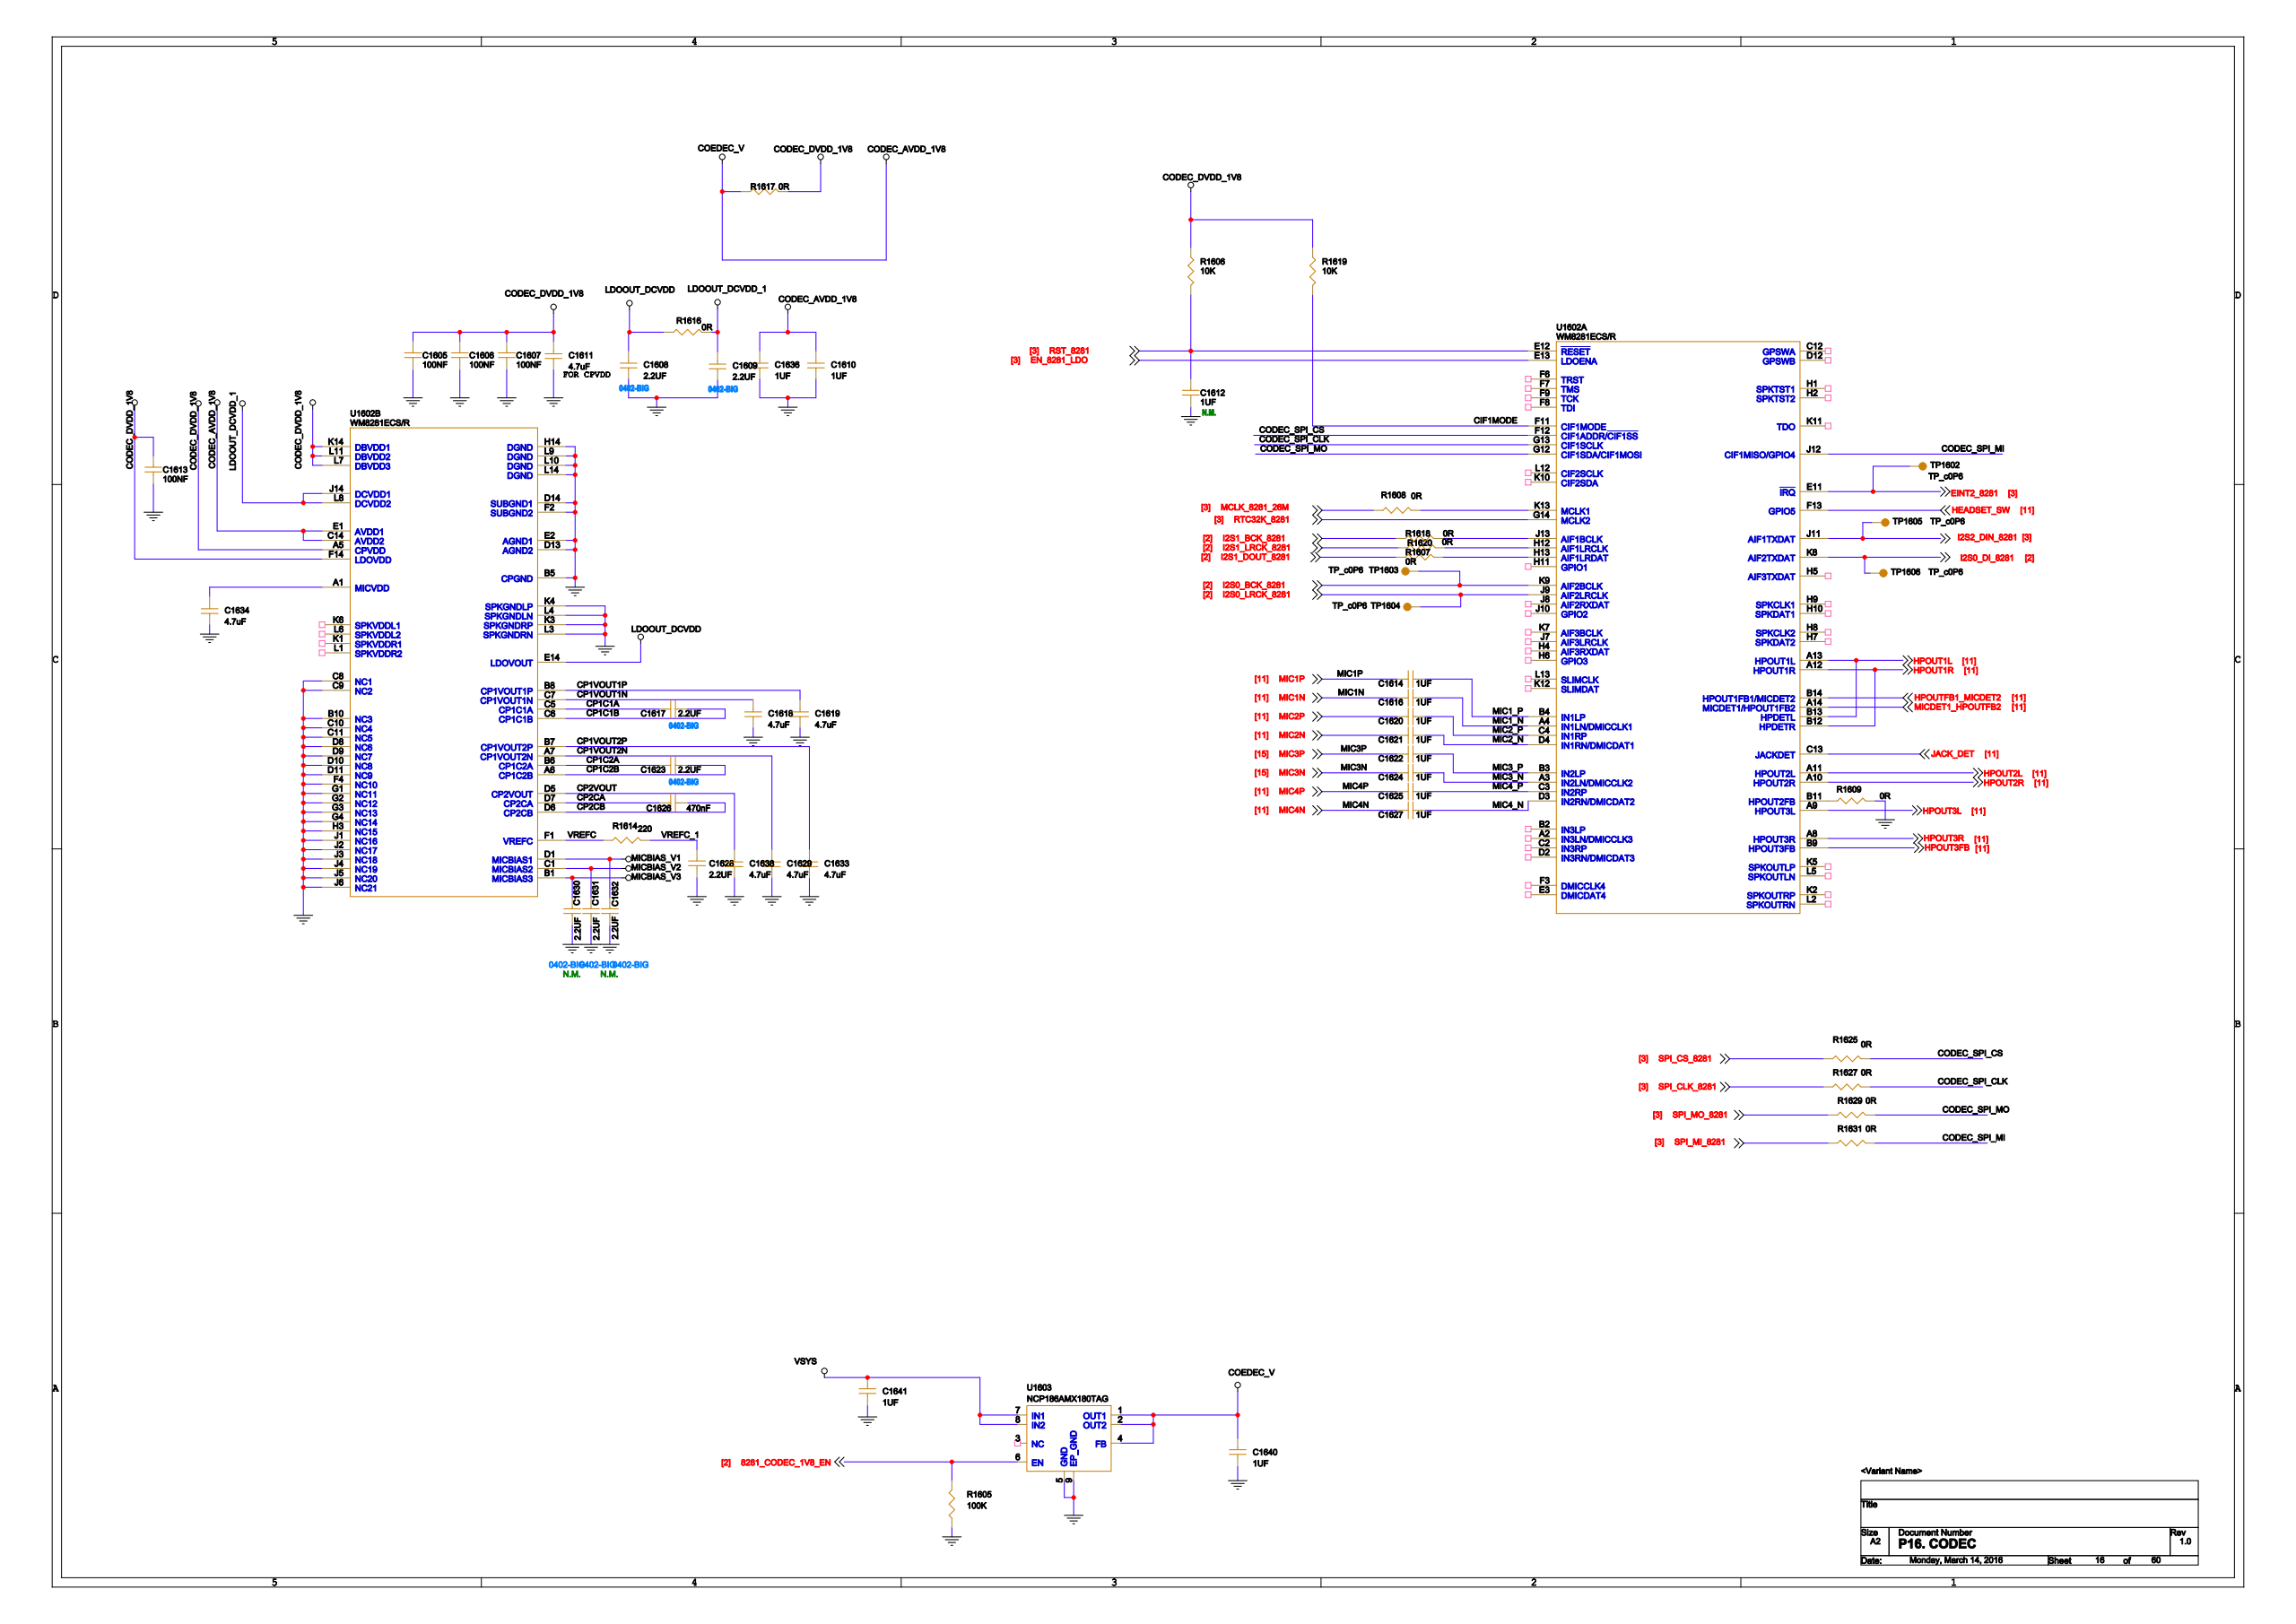Circuit board | Cadence Allegro | 1088 parts | 793 nets | one sheet of the schematic
Parts on this sheet (reference | value | footprint):
C1605 | 100NF | C0201
C1606 | 100NF | C0201
C1607 | 100NF | C0201
C1608 | 2.2UF | 0402-BIG
C1609 | 2.2UF | 0402-BIG
C1610 | 1UF | C0201
C1611 | 4.7uF | 0402-BIG
C1612
C1613 | 100NF | C0201
C1614 | 1UF | C0201
C1616 | 1UF | C0201
C1617 | 2.2UF | 0402-BIG
C1618 | 4.7uF | 0402-BIG
C1619 | 4.7uF | 0402-BIG
C1620 | 1UF | C0201
C1621 | 1UF | C0201
C1622 | 1UF | C0201
C1623 | 2.2UF | 0402-BIG
C1624 | 1UF | C0201
C1625 | 1UF | C0201
C1626 | 470nF | C0201
C1627 | 1UF | C0201
C1628 | 2.2UF | 0402-BIG
C1629 | 4.7uF | 0402-BIG
C1630
C1631 | 2.2UF | 0402-BIG
C1632
C1633 | 4.7uF | 0402-BIG
C1634 | 4.7uF | 0402-BIG
C1636 | 1UF | C0201
C1638 | 4.7uF | 0402-BIG
C1640 | 1UF | C0201
C1641 | 1UF | C0201
R1605 | 100K | R0201
R1606 | 10K | R0201
R1607 | 0R | R0201
R1608 | 0R | R0201
R1609 | 0R | R0201
R1616 | 0R | R0201
R1617 | 0R | R0201
R1618 | 0R | R0201
R1619 | 10K | R0201
R1620 | 0R | R0201
R1625 | 0R | R0201
R1627 | 0R | R0201
R1629 | 0R | R0201
R1631 | 0R | R0201
TP1602 | TP_c0P6 | TP_C0P6
TP1603 | TP_c0P6 | TP_C0P6
TP1604 | TP_c0P6 | TP_C0P6
TP1605 | TP_c0P6 | TP_C0P6
TP1606 | TP_c0P6 | TP_C0P6
U1602 | WM8281ECS/R | WCSP138_4P555X5P855X0P781_0P4
U1603 | NCP186AMX180TAG | XDFN8_1P2X1P6X0P55_0P4
Nets of these parts (net: part-pin ...):
GND: C1605-2 C1606-2 C1607-2 C1608-1 C1609-1 C1610-1 C1611-1 C1612-2 C1613-2 C1618-1 C1619-1 C1628-2 C1629-1 C1630-2 C1631-2 C1632-2 C1633-1 C1634-1 C1636-1 C1638-1 C1640-2 C1641-2 R1605-1 R1609-2 U1603-5 U1603-9 U1602-B5 U1602-B10 U1602-C8 U1602-C9 U1602-C10 U1602-C11 U1602-D8 U1602-D9 U1602-D10 U1602-D11 U1602-D13 U1602-D14 U1602-E2 U1602-F2 U1602-F4 U1602-G1 U1602-G2 U1602-G3 U1602-G4 U1602-H3 U1602-H14 U1602-J1 U1602-J2 U1602-J3 U1602-J4 U1602-J5 U1602-J6 U1602-K3 U1602-K4 U1602-L3 U1602-L4 U1602-L9 U1602-L10 U1602-L14
VSYS: C1641-1 U1603-7 U1603-8
MIC4P: C1625-1
MICBIAS_V2: C1631-1 U1602-C1
MIC1P: C1614-1
8281_CODEC_1V8_EN: R1605-2 U1603-6
I2S1_LRCK_8281: R1620-1
I2S1_DOUT_8281: R1607-1
EINT2_8281: TP1602-1 U1602-E11
I2S0_LRCK_8281: TP1604-1 U1602-J9
I2S0_BCK_8281: TP1603-1 U1602-K9
I2S2_DIN_8281: TP1605-1 U1602-J11
I2S1_BCK_8281: R1618-1
SPI_CLK_8281: R1627-1
EN_8281_LDO: U1602-E13
SPI_MO_8281: R1629-1
SPI_MI_8281: R1631-1
SPI_CS_8281: R1625-1
MCLK_8281_26M: R1608-1
RST_8281: C1612-1 R1606-2 U1602-E12
I2S0_DI_8281: TP1606-1 U1602-K8
HPOUT2L: U1602-A11
HPOUT2R: U1602-A10
HPOUT1L: U1602-A13 U1602-B13
HPOUT1R: U1602-A12 U1602-B12
VREFC: U1602-F1
VREFC_1: C1628-1
N34980372: R1618-2 U1602-J13
N34980384: R1620-2 U1602-H12
N34980407: R1607-2 U1602-H13
CODEC_SPI_CS: R1625-2 U1602-F12
CODEC_SPI_MI: R1631-2 U1602-J12
CIF1MODE: R1619-2 U1602-F11
CODEC_SPI_CLK: R1627-2 U1602-G13
CODEC_SPI_MO: R1629-2 U1602-G12
HEADSET_SW: U1602-F13
HPOUTFB1_MICDET2: U1602-B14
N3458626166: R1609-1 U1602-B11
HPOUT3FB: U1602-B9
HPOUT3L: U1602-A9
HPOUT3R: U1602-A8
MIC1_N: C1616-2 U1602-A4
MIC1_P: C1614-2 U1602-B4
MIC2_N: C1621-2 U1602-D4
MIC2_P: C1620-2 U1602-C4
MIC3_N: C1624-2 U1602-A3
MIC3_P: C1622-2 U1602-B3
MIC4_N: C1627-2 U1602-D3
MIC4_P: C1625-2 U1602-C3
JACK_DET: U1602-C13
N18434224: R1608-2 U1602-K13
RTC32K_8281: U1602-G14
MICDET1_HPOUTFB2: U1602-A14
CODEC_AVDD_1V8: C1610-2 C1636-2 C1640-1 R1617-1 U1603-1 U1603-2 U1603-4 U1602-C14 U1602-E1
CP1C1A: C1617-1 U1602-C5
CP1C1B: C1617-2 U1602-C6
CP1C2A: C1623-1 U1602-B6
CP1C2B: C1623-2 U1602-A6
CP1VOUT1N: C1618-2 U1602-C7
CP1VOUT1P: C1619-2 U1602-B8
CP1VOUT2N: C1629-2 U1602-A7
CP1VOUT2P: C1633-2 U1602-B7
CP2CA: C1626-1 U1602-D7
CP2CB: C1626-2 U1602-D6
CP2VOUT: C1638-2 U1602-D5
CODEC_DVDD_1V8: C1605-1 C1606-1 C1607-1 C1611-2 C1613-1 R1606-1 R1617-2 R1619-1 U1602-A5 U1602-F14 U1602-K14 U1602-L7 U1602-L11
LDOOUT_DCVDD_1: C1609-2 R1616-2 U1602-J14 U1602-L8
LDOOUT_DCVDD: C1608-2 R1616-1 U1602-E14
MICBIAS_V1: C1632-1 U1602-D1
MICBIAS_V3: C1630-1 U1602-B1
N17697439: C1634-2 U1602-A1
MIC1N: C1616-1
MIC2P: C1620-1
MIC2N: C1621-1
MIC3P: C1622-1
MIC3N: C1624-1
MIC4N: C1627-1